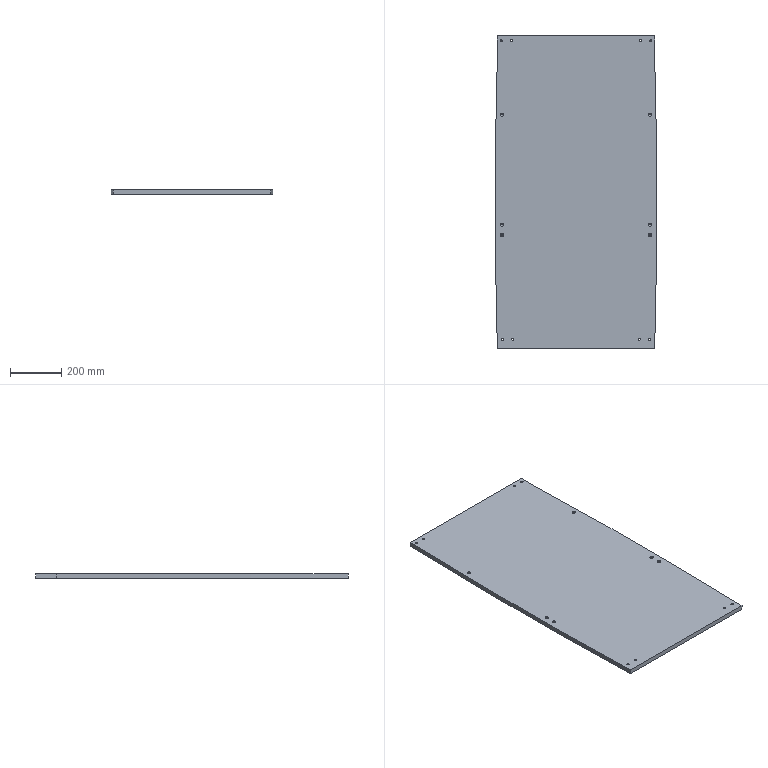Part | STEP file | DECAK 615 | 1 solid | 28 faces | box 633 x 1220 x 18 mm | volume 13739057 mm3 | cylinder 16 | plane 6 | cone 6 | commonest cylinder face diameters 8.5 x8 6.6 x6 36109 x2
STEP:
#1=CARTESIAN_POINT('',(307.5,530.,9.));
#2=VERTEX_POINT('',#1);
#3=CARTESIAN_POINT('',(307.5,610.,9.));
#4=VERTEX_POINT('',#3);
#5=CARTESIAN_POINT('',(307.5,610.,9.));
#6=DIRECTION('',(0.,1.,0.));
#7=VECTOR('',#6,1000.);
#8=LINE('',#5,#7);
#9=EDGE_CURVE('',#2,#4,#8,.T.);
#10=ORIENTED_EDGE('',*,*,#9,.F.);
#11=CARTESIAN_POINT('',(307.5,530.,-9.));
#12=VERTEX_POINT('',#11);
#13=CARTESIAN_POINT('',(307.5,530.,-1149.086));
#14=DIRECTION('',(0.,0.,1.));
#15=VECTOR('',#14,1000.);
#16=LINE('',#13,#15);
#17=EDGE_CURVE('',#12,#2,#16,.T.);
#18=ORIENTED_EDGE('',*,*,#17,.F.);
#19=CARTESIAN_POINT('',(307.5,610.,-9.));
#20=VERTEX_POINT('',#19);
#21=CARTESIAN_POINT('',(307.5,610.,-9.));
#22=DIRECTION('',(0.,1.,0.));
#23=VECTOR('',#22,1000.);
#24=LINE('',#21,#23);
#25=EDGE_CURVE('',#12,#20,#24,.T.);
#26=ORIENTED_EDGE('',*,*,#25,.T.);
#27=CARTESIAN_POINT('',(307.5,610.,9.));
#28=DIRECTION('',(0.,0.,-1.));
#29=VECTOR('',#28,1000.);
#30=LINE('',#27,#29);
#31=EDGE_CURVE('',#4,#20,#30,.T.);
#32=ORIENTED_EDGE('',*,*,#31,.F.);
#33=EDGE_LOOP('',(#10,#18,#26,#32));
#34=FACE_OUTER_BOUND('',#33,.T.);
#35=CARTESIAN_POINT('',(307.5,610.,9.));
#36=DIRECTION('',(-1.,0.,0.));
#37=DIRECTION('',(0.,0.,1.));
#38=AXIS2_PLACEMENT_3D('',#35,#36,#37);
#39=PLANE('',#38);
#40=ADVANCED_FACE('',(#34),#39,.F.);
#41=CARTESIAN_POINT('',(-307.5,610.,-9.));
#42=VERTEX_POINT('',#41);
#43=CARTESIAN_POINT('',(-307.5,610.,-9.));
#44=DIRECTION('',(-1.,0.,0.));
#45=VECTOR('',#44,1000.);
#46=LINE('',#43,#45);
#47=EDGE_CURVE('',#20,#42,#46,.T.);
#48=ORIENTED_EDGE('',*,*,#47,.T.);
#49=CARTESIAN_POINT('',(-307.5,610.,9.));
#50=VERTEX_POINT('',#49);
#51=CARTESIAN_POINT('',(-307.5,610.,9.));
#52=DIRECTION('',(0.,0.,-1.));
#53=VECTOR('',#52,1000.);
#54=LINE('',#51,#53);
#55=EDGE_CURVE('',#50,#42,#54,.T.);
#56=ORIENTED_EDGE('',*,*,#55,.F.);
#57=CARTESIAN_POINT('',(-307.5,610.,9.));
#58=DIRECTION('',(-1.,0.,0.));
#59=VECTOR('',#58,1000.);
#60=LINE('',#57,#59);
#61=EDGE_CURVE('',#4,#50,#60,.T.);
#62=ORIENTED_EDGE('',*,*,#61,.F.);
#63=ORIENTED_EDGE('',*,*,#31,.T.);
#64=EDGE_LOOP('',(#48,#56,#62,#63));
#65=FACE_OUTER_BOUND('',#64,.T.);
#66=CARTESIAN_POINT('',(-307.5,610.,9.));
#67=DIRECTION('',(0.,-1.,0.));
#68=DIRECTION('',(1.,0.,0.));
#69=AXIS2_PLACEMENT_3D('',#66,#67,#68);
#70=PLANE('',#69);
#71=ADVANCED_FACE('',(#65),#70,.F.);
#72=CARTESIAN_POINT('',(-307.5,530.,-9.));
#73=VERTEX_POINT('',#72);
#74=CARTESIAN_POINT('',(-307.5,610.,-9.));
#75=DIRECTION('',(0.,-1.,0.));
#76=VECTOR('',#75,1000.);
#77=LINE('',#74,#76);
#78=EDGE_CURVE('',#42,#73,#77,.T.);
#79=ORIENTED_EDGE('',*,*,#78,.T.);
#80=CARTESIAN_POINT('',(-307.5,530.,9.));
#81=VERTEX_POINT('',#80);
#82=CARTESIAN_POINT('',(-307.5,530.,-1149.086));
#83=DIRECTION('',(0.,0.,1.));
#84=VECTOR('',#83,1000.);
#85=LINE('',#82,#84);
#86=EDGE_CURVE('',#73,#81,#85,.T.);
#87=ORIENTED_EDGE('',*,*,#86,.T.);
#88=CARTESIAN_POINT('',(-307.5,610.,9.));
#89=DIRECTION('',(0.,-1.,0.));
#90=VECTOR('',#89,1000.);
#91=LINE('',#88,#90);
#92=EDGE_CURVE('',#50,#81,#91,.T.);
#93=ORIENTED_EDGE('',*,*,#92,.F.);
#94=ORIENTED_EDGE('',*,*,#55,.T.);
#95=EDGE_LOOP('',(#79,#87,#93,#94));
#96=FACE_OUTER_BOUND('',#95,.T.);
#97=CARTESIAN_POINT('',(-307.5,610.,9.));
#98=DIRECTION('',(1.,0.,0.));
#99=DIRECTION('',(0.,0.,-1.));
#100=AXIS2_PLACEMENT_3D('',#97,#98,#99);
#101=PLANE('',#100);
#102=ADVANCED_FACE('',(#96),#101,.F.);
#103=CARTESIAN_POINT('',(-307.5,-610.,-9.));
#104=VERTEX_POINT('',#103);
#105=CARTESIAN_POINT('',(307.5,-610.,-9.));
#106=VERTEX_POINT('',#105);
#107=CARTESIAN_POINT('',(-307.5,-610.,-9.));
#108=DIRECTION('',(1.,0.,0.));
#109=VECTOR('',#108,1000.);
#110=LINE('',#107,#109);
#111=EDGE_CURVE('',#104,#106,#110,.T.);
#112=ORIENTED_EDGE('',*,*,#111,.T.);
#113=CARTESIAN_POINT('',(307.5,-610.,9.));
#114=VERTEX_POINT('',#113);
#115=CARTESIAN_POINT('',(307.5,-610.,9.));
#116=DIRECTION('',(0.,0.,-1.));
#117=VECTOR('',#116,1000.);
#118=LINE('',#115,#117);
#119=EDGE_CURVE('',#114,#106,#118,.T.);
#120=ORIENTED_EDGE('',*,*,#119,.F.);
#121=CARTESIAN_POINT('',(-307.5,-610.,9.));
#122=VERTEX_POINT('',#121);
#123=CARTESIAN_POINT('',(-307.5,-610.,9.));
#124=DIRECTION('',(1.,0.,0.));
#125=VECTOR('',#124,1000.);
#126=LINE('',#123,#125);
#127=EDGE_CURVE('',#122,#114,#126,.T.);
#128=ORIENTED_EDGE('',*,*,#127,.F.);
#129=CARTESIAN_POINT('',(-307.5,-610.,9.));
#130=DIRECTION('',(0.,0.,-1.));
#131=VECTOR('',#130,1000.);
#132=LINE('',#129,#131);
#133=EDGE_CURVE('',#122,#104,#132,.T.);
#134=ORIENTED_EDGE('',*,*,#133,.T.);
#135=EDGE_LOOP('',(#112,#120,#128,#134));
#136=FACE_OUTER_BOUND('',#135,.T.);
#137=CARTESIAN_POINT('',(-307.5,-610.,9.));
#138=DIRECTION('',(0.,1.,0.));
#139=DIRECTION('',(-1.,0.,0.));
#140=AXIS2_PLACEMENT_3D('',#137,#138,#139);
#141=PLANE('',#140);
#142=ADVANCED_FACE('',(#136),#141,.F.);
#143=CARTESIAN_POINT('',(288.25,591.,9.));
#144=VERTEX_POINT('',#143);
#145=CARTESIAN_POINT('',(292.5,591.,9.));
#146=DIRECTION('',(0.,0.,1.));
#147=DIRECTION('',(-1.,0.,0.));
#148=AXIS2_PLACEMENT_3D('',#145,#146,#147);
#149=CIRCLE('',#148,4.25);
#150=EDGE_CURVE('',#144,#144,#149,.T.);
#151=ORIENTED_EDGE('',*,*,#150,.F.);
#152=EDGE_LOOP('',(#151));
#153=FACE_BOUND('',#152,.T.);
#154=CARTESIAN_POINT('',(248.25,591.,9.));
#155=VERTEX_POINT('',#154);
#156=CARTESIAN_POINT('',(252.5,591.,9.));
#157=DIRECTION('',(0.,0.,1.));
#158=DIRECTION('',(-1.,0.,0.));
#159=AXIS2_PLACEMENT_3D('',#156,#157,#158);
#160=CIRCLE('',#159,4.25);
#161=EDGE_CURVE('',#155,#155,#160,.T.);
#162=ORIENTED_EDGE('',*,*,#161,.F.);
#163=EDGE_LOOP('',(#162));
#164=FACE_BOUND('',#163,.T.);
#165=CARTESIAN_POINT('',(-248.25,591.,9.));
#166=VERTEX_POINT('',#165);
#167=CARTESIAN_POINT('',(-252.5,591.,9.));
#168=DIRECTION('',(0.,0.,1.));
#169=DIRECTION('',(1.,0.,0.));
#170=AXIS2_PLACEMENT_3D('',#167,#168,#169);
#171=CIRCLE('',#170,4.25);
#172=EDGE_CURVE('',#166,#166,#171,.T.);
#173=ORIENTED_EDGE('',*,*,#172,.F.);
#174=EDGE_LOOP('',(#173));
#175=FACE_BOUND('',#174,.T.);
#176=CARTESIAN_POINT('',(-288.25,591.,9.));
#177=VERTEX_POINT('',#176);
#178=CARTESIAN_POINT('',(-292.5,591.,9.));
#179=DIRECTION('',(0.,0.,1.));
#180=DIRECTION('',(1.,0.,0.));
#181=AXIS2_PLACEMENT_3D('',#178,#179,#180);
#182=CIRCLE('',#181,4.25);
#183=EDGE_CURVE('',#177,#177,#182,.T.);
#184=ORIENTED_EDGE('',*,*,#183,.F.);
#185=EDGE_LOOP('',(#184));
#186=FACE_BOUND('',#185,.T.);
#187=CARTESIAN_POINT('',(283.25,-575.,9.));
#188=VERTEX_POINT('',#187);
#189=CARTESIAN_POINT('',(287.5,-575.,9.));
#190=DIRECTION('',(0.,0.,1.));
#191=DIRECTION('',(-1.,0.,0.));
#192=AXIS2_PLACEMENT_3D('',#189,#190,#191);
#193=CIRCLE('',#192,4.25);
#194=EDGE_CURVE('',#188,#188,#193,.T.);
#195=ORIENTED_EDGE('',*,*,#194,.F.);
#196=EDGE_LOOP('',(#195));
#197=FACE_BOUND('',#196,.T.);
#198=CARTESIAN_POINT('',(243.25,-575.,9.));
#199=VERTEX_POINT('',#198);
#200=CARTESIAN_POINT('',(247.5,-575.,9.));
#201=DIRECTION('',(0.,0.,1.));
#202=DIRECTION('',(-1.,0.,0.));
#203=AXIS2_PLACEMENT_3D('',#200,#201,#202);
#204=CIRCLE('',#203,4.25);
#205=EDGE_CURVE('',#199,#199,#204,.T.);
#206=ORIENTED_EDGE('',*,*,#205,.F.);
#207=EDGE_LOOP('',(#206));
#208=FACE_BOUND('',#207,.T.);
#209=CARTESIAN_POINT('',(-243.25,-575.,9.));
#210=VERTEX_POINT('',#209);
#211=CARTESIAN_POINT('',(-247.5,-575.,9.));
#212=DIRECTION('',(0.,0.,1.));
#213=DIRECTION('',(1.,0.,0.));
#214=AXIS2_PLACEMENT_3D('',#211,#212,#213);
#215=CIRCLE('',#214,4.25);
#216=EDGE_CURVE('',#210,#210,#215,.T.);
#217=ORIENTED_EDGE('',*,*,#216,.F.);
#218=EDGE_LOOP('',(#217));
#219=FACE_BOUND('',#218,.T.);
#220=CARTESIAN_POINT('',(-283.25,-575.,9.));
#221=VERTEX_POINT('',#220);
#222=CARTESIAN_POINT('',(-287.5,-575.,9.));
#223=DIRECTION('',(0.,0.,1.));
#224=DIRECTION('',(1.,0.,0.));
#225=AXIS2_PLACEMENT_3D('',#222,#223,#224);
#226=CIRCLE('',#225,4.25);
#227=EDGE_CURVE('',#221,#221,#226,.T.);
#228=ORIENTED_EDGE('',*,*,#227,.F.);
#229=EDGE_LOOP('',(#228));
#230=FACE_BOUND('',#229,.T.);
#231=ORIENTED_EDGE('',*,*,#127,.T.);
#232=CARTESIAN_POINT('',(-17738.,-40.,9.));
#233=DIRECTION('',(0.,0.,1.));
#234=DIRECTION('',(-1.,0.,0.));
#235=AXIS2_PLACEMENT_3D('',#232,#233,#234);
#236=CIRCLE('',#235,18054.5);
#237=EDGE_CURVE('',#114,#2,#236,.T.);
#238=ORIENTED_EDGE('',*,*,#237,.T.);
#239=ORIENTED_EDGE('',*,*,#9,.T.);
#240=ORIENTED_EDGE('',*,*,#61,.T.);
#241=ORIENTED_EDGE('',*,*,#92,.T.);
#242=CARTESIAN_POINT('',(17738.,-40.,9.));
#243=DIRECTION('',(0.,0.,1.));
#244=DIRECTION('',(1.,0.,0.));
#245=AXIS2_PLACEMENT_3D('',#242,#243,#244);
#246=CIRCLE('',#245,18054.5);
#247=EDGE_CURVE('',#81,#122,#246,.T.);
#248=ORIENTED_EDGE('',*,*,#247,.T.);
#249=EDGE_LOOP('',(#231,#238,#239,#240,#241,#248));
#250=FACE_OUTER_BOUND('',#249,.T.);
#251=CARTESIAN_POINT('',(295.8,-168.,9.));
#252=VERTEX_POINT('',#251);
#253=CARTESIAN_POINT('',(289.5,-168.,9.));
#254=DIRECTION('',(0.,0.,-1.));
#255=DIRECTION('',(1.,0.,0.));
#256=AXIS2_PLACEMENT_3D('',#253,#254,#255);
#257=CIRCLE('',#256,6.3);
#258=EDGE_CURVE('',#252,#252,#257,.T.);
#259=ORIENTED_EDGE('',*,*,#258,.T.);
#260=EDGE_LOOP('',(#259));
#261=FACE_BOUND('',#260,.T.);
#262=CARTESIAN_POINT('',(-283.2,-168.,9.));
#263=VERTEX_POINT('',#262);
#264=CARTESIAN_POINT('',(-289.5,-168.,9.));
#265=DIRECTION('',(0.,0.,-1.));
#266=DIRECTION('',(1.,0.,0.));
#267=AXIS2_PLACEMENT_3D('',#264,#265,#266);
#268=CIRCLE('',#267,6.3);
#269=EDGE_CURVE('',#263,#263,#268,.T.);
#270=ORIENTED_EDGE('',*,*,#269,.T.);
#271=EDGE_LOOP('',(#270));
#272=FACE_BOUND('',#271,.T.);
#273=CARTESIAN_POINT('',(295.8,-128.,9.));
#274=VERTEX_POINT('',#273);
#275=CARTESIAN_POINT('',(289.5,-128.,9.));
#276=DIRECTION('',(0.,0.,-1.));
#277=DIRECTION('',(1.,0.,0.));
#278=AXIS2_PLACEMENT_3D('',#275,#276,#277);
#279=CIRCLE('',#278,6.3);
#280=EDGE_CURVE('',#274,#274,#279,.T.);
#281=ORIENTED_EDGE('',*,*,#280,.T.);
#282=EDGE_LOOP('',(#281));
#283=FACE_BOUND('',#282,.T.);
#284=CARTESIAN_POINT('',(295.8,302.,9.));
#285=VERTEX_POINT('',#284);
#286=CARTESIAN_POINT('',(289.5,302.,9.));
#287=DIRECTION('',(0.,0.,-1.));
#288=DIRECTION('',(1.,0.,0.));
#289=AXIS2_PLACEMENT_3D('',#286,#287,#288);
#290=CIRCLE('',#289,6.3);
#291=EDGE_CURVE('',#285,#285,#290,.T.);
#292=ORIENTED_EDGE('',*,*,#291,.T.);
#293=EDGE_LOOP('',(#292));
#294=FACE_BOUND('',#293,.T.);
#295=CARTESIAN_POINT('',(-283.2,-128.,9.));
#296=VERTEX_POINT('',#295);
#297=CARTESIAN_POINT('',(-289.5,-128.,9.));
#298=DIRECTION('',(0.,0.,-1.));
#299=DIRECTION('',(1.,0.,0.));
#300=AXIS2_PLACEMENT_3D('',#297,#298,#299);
#301=CIRCLE('',#300,6.3);
#302=EDGE_CURVE('',#296,#296,#301,.T.);
#303=ORIENTED_EDGE('',*,*,#302,.T.);
#304=EDGE_LOOP('',(#303));
#305=FACE_BOUND('',#304,.T.);
#306=CARTESIAN_POINT('',(-283.2,302.,9.));
#307=VERTEX_POINT('',#306);
#308=CARTESIAN_POINT('',(-289.5,302.,9.));
#309=DIRECTION('',(0.,0.,-1.));
#310=DIRECTION('',(1.,0.,0.));
#311=AXIS2_PLACEMENT_3D('',#308,#309,#310);
#312=CIRCLE('',#311,6.3);
#313=EDGE_CURVE('',#307,#307,#312,.T.);
#314=ORIENTED_EDGE('',*,*,#313,.T.);
#315=EDGE_LOOP('',(#314));
#316=FACE_BOUND('',#315,.T.);
#317=CARTESIAN_POINT('',(307.5,-610.,9.));
#318=DIRECTION('',(0.,0.,1.));
#319=DIRECTION('',(1.,0.,0.));
#320=AXIS2_PLACEMENT_3D('',#317,#318,#319);
#321=PLANE('',#320);
#322=ADVANCED_FACE('',(#153,#164,#175,#186,#197,#208,#219,#230,#250,#261,#272,#283,#294,#305,#316),#321,.T.);
#323=CARTESIAN_POINT('',(288.25,591.,-9.));
#324=VERTEX_POINT('',#323);
#325=CARTESIAN_POINT('',(292.5,591.,-9.));
#326=DIRECTION('',(0.,0.,1.));
#327=DIRECTION('',(-1.,0.,0.));
#328=AXIS2_PLACEMENT_3D('',#325,#326,#327);
#329=CIRCLE('',#328,4.25);
#330=EDGE_CURVE('',#324,#324,#329,.T.);
#331=ORIENTED_EDGE('',*,*,#330,.T.);
#332=EDGE_LOOP('',(#331));
#333=FACE_BOUND('',#332,.T.);
#334=CARTESIAN_POINT('',(248.25,591.,-9.));
#335=VERTEX_POINT('',#334);
#336=CARTESIAN_POINT('',(252.5,591.,-9.));
#337=DIRECTION('',(0.,0.,1.));
#338=DIRECTION('',(-1.,0.,0.));
#339=AXIS2_PLACEMENT_3D('',#336,#337,#338);
#340=CIRCLE('',#339,4.25);
#341=EDGE_CURVE('',#335,#335,#340,.T.);
#342=ORIENTED_EDGE('',*,*,#341,.T.);
#343=EDGE_LOOP('',(#342));
#344=FACE_BOUND('',#343,.T.);
#345=CARTESIAN_POINT('',(-248.25,591.,-9.));
#346=VERTEX_POINT('',#345);
#347=CARTESIAN_POINT('',(-252.5,591.,-9.));
#348=DIRECTION('',(0.,0.,1.));
#349=DIRECTION('',(1.,0.,0.));
#350=AXIS2_PLACEMENT_3D('',#347,#348,#349);
#351=CIRCLE('',#350,4.25);
#352=EDGE_CURVE('',#346,#346,#351,.T.);
#353=ORIENTED_EDGE('',*,*,#352,.T.);
#354=EDGE_LOOP('',(#353));
#355=FACE_BOUND('',#354,.T.);
#356=CARTESIAN_POINT('',(-288.25,591.,-9.));
#357=VERTEX_POINT('',#356);
#358=CARTESIAN_POINT('',(-292.5,591.,-9.));
#359=DIRECTION('',(0.,0.,1.));
#360=DIRECTION('',(1.,0.,0.));
#361=AXIS2_PLACEMENT_3D('',#358,#359,#360);
#362=CIRCLE('',#361,4.25);
#363=EDGE_CURVE('',#357,#357,#362,.T.);
#364=ORIENTED_EDGE('',*,*,#363,.T.);
#365=EDGE_LOOP('',(#364));
#366=FACE_BOUND('',#365,.T.);
#367=CARTESIAN_POINT('',(283.25,-575.,-9.));
#368=VERTEX_POINT('',#367);
#369=CARTESIAN_POINT('',(287.5,-575.,-9.));
#370=DIRECTION('',(0.,0.,1.));
#371=DIRECTION('',(-1.,0.,0.));
#372=AXIS2_PLACEMENT_3D('',#369,#370,#371);
#373=CIRCLE('',#372,4.25);
#374=EDGE_CURVE('',#368,#368,#373,.T.);
#375=ORIENTED_EDGE('',*,*,#374,.T.);
#376=EDGE_LOOP('',(#375));
#377=FACE_BOUND('',#376,.T.);
#378=CARTESIAN_POINT('',(243.25,-575.,-9.));
#379=VERTEX_POINT('',#378);
#380=CARTESIAN_POINT('',(247.5,-575.,-9.));
#381=DIRECTION('',(0.,0.,1.));
#382=DIRECTION('',(-1.,0.,0.));
#383=AXIS2_PLACEMENT_3D('',#380,#381,#382);
#384=CIRCLE('',#383,4.25);
#385=EDGE_CURVE('',#379,#379,#384,.T.);
#386=ORIENTED_EDGE('',*,*,#385,.T.);
#387=EDGE_LOOP('',(#386));
#388=FACE_BOUND('',#387,.T.);
#389=CARTESIAN_POINT('',(-243.25,-575.,-9.));
#390=VERTEX_POINT('',#389);
#391=CARTESIAN_POINT('',(-247.5,-575.,-9.));
#392=DIRECTION('',(0.,0.,1.));
#393=DIRECTION('',(1.,0.,0.));
#394=AXIS2_PLACEMENT_3D('',#391,#392,#393);
#395=CIRCLE('',#394,4.25);
#396=EDGE_CURVE('',#390,#390,#395,.T.);
#397=ORIENTED_EDGE('',*,*,#396,.T.);
#398=EDGE_LOOP('',(#397));
#399=FACE_BOUND('',#398,.T.);
#400=CARTESIAN_POINT('',(-283.25,-575.,-9.));
#401=VERTEX_POINT('',#400);
#402=CARTESIAN_POINT('',(-287.5,-575.,-9.));
#403=DIRECTION('',(0.,0.,1.));
#404=DIRECTION('',(1.,0.,0.));
#405=AXIS2_PLACEMENT_3D('',#402,#403,#404);
#406=CIRCLE('',#405,4.25);
#407=EDGE_CURVE('',#401,#401,#406,.T.);
#408=ORIENTED_EDGE('',*,*,#407,.T.);
#409=EDGE_LOOP('',(#408));
#410=FACE_BOUND('',#409,.T.);
#411=CARTESIAN_POINT('',(-17738.,-40.,-9.));
#412=DIRECTION('',(0.,0.,-1.));
#413=DIRECTION('',(1.,0.,0.));
#414=AXIS2_PLACEMENT_3D('',#411,#412,#413);
#415=CIRCLE('',#414,18054.5);
#416=EDGE_CURVE('',#12,#106,#415,.T.);
#417=ORIENTED_EDGE('',*,*,#416,.T.);
#418=ORIENTED_EDGE('',*,*,#111,.F.);
#419=CARTESIAN_POINT('',(17738.,-40.,-9.));
#420=DIRECTION('',(0.,0.,-1.));
#421=DIRECTION('',(1.,0.,0.));
#422=AXIS2_PLACEMENT_3D('',#419,#420,#421);
#423=CIRCLE('',#422,18054.5);
#424=EDGE_CURVE('',#104,#73,#423,.T.);
#425=ORIENTED_EDGE('',*,*,#424,.T.);
#426=ORIENTED_EDGE('',*,*,#78,.F.);
#427=ORIENTED_EDGE('',*,*,#47,.F.);
#428=ORIENTED_EDGE('',*,*,#25,.F.);
#429=EDGE_LOOP('',(#417,#418,#425,#426,#427,#428));
#430=FACE_OUTER_BOUND('',#429,.T.);
#431=CARTESIAN_POINT('',(286.2,-168.,-9.));
#432=VERTEX_POINT('',#431);
#433=CARTESIAN_POINT('',(289.5,-168.,-9.));
#434=DIRECTION('',(0.,0.,1.));
#435=DIRECTION('',(-1.,0.,0.));
#436=AXIS2_PLACEMENT_3D('',#433,#434,#435);
#437=CIRCLE('',#436,3.3);
#438=EDGE_CURVE('',#432,#432,#437,.T.);
#439=ORIENTED_EDGE('',*,*,#438,.T.);
#440=EDGE_LOOP('',(#439));
#441=FACE_BOUND('',#440,.T.);
#442=CARTESIAN_POINT('',(286.2,302.,-9.));
#443=VERTEX_POINT('',#442);
#444=CARTESIAN_POINT('',(289.5,302.,-9.));
#445=DIRECTION('',(0.,0.,1.));
#446=DIRECTION('',(-1.,0.,0.));
#447=AXIS2_PLACEMENT_3D('',#444,#445,#446);
#448=CIRCLE('',#447,3.3);
#449=EDGE_CURVE('',#443,#443,#448,.T.);
#450=ORIENTED_EDGE('',*,*,#449,.T.);
#451=EDGE_LOOP('',(#450));
#452=FACE_BOUND('',#451,.T.);
#453=CARTESIAN_POINT('',(286.2,-128.,-9.));
#454=VERTEX_POINT('',#453);
#455=CARTESIAN_POINT('',(289.5,-128.,-9.));
#456=DIRECTION('',(0.,0.,1.));
#457=DIRECTION('',(-1.,0.,0.));
#458=AXIS2_PLACEMENT_3D('',#455,#456,#457);
#459=CIRCLE('',#458,3.3);
#460=EDGE_CURVE('',#454,#454,#459,.T.);
#461=ORIENTED_EDGE('',*,*,#460,.T.);
#462=EDGE_LOOP('',(#461));
#463=FACE_BOUND('',#462,.T.);
#464=CARTESIAN_POINT('',(-286.2,-168.,-9.));
#465=VERTEX_POINT('',#464);
#466=CARTESIAN_POINT('',(-289.5,-168.,-9.));
#467=DIRECTION('',(0.,0.,1.));
#468=DIRECTION('',(1.,0.,0.));
#469=AXIS2_PLACEMENT_3D('',#466,#467,#468);
#470=CIRCLE('',#469,3.3);
#471=EDGE_CURVE('',#465,#465,#470,.T.);
#472=ORIENTED_EDGE('',*,*,#471,.T.);
#473=EDGE_LOOP('',(#472));
#474=FACE_BOUND('',#473,.T.);
#475=CARTESIAN_POINT('',(-286.2,-128.,-9.));
#476=VERTEX_POINT('',#475);
#477=CARTESIAN_POINT('',(-289.5,-128.,-9.));
#478=DIRECTION('',(0.,0.,1.));
#479=DIRECTION('',(1.,0.,0.));
#480=AXIS2_PLACEMENT_3D('',#477,#478,#479);
#481=CIRCLE('',#480,3.3);
#482=EDGE_CURVE('',#476,#476,#481,.T.);
#483=ORIENTED_EDGE('',*,*,#482,.T.);
#484=EDGE_LOOP('',(#483));
#485=FACE_BOUND('',#484,.T.);
#486=CARTESIAN_POINT('',(-286.2,302.,-9.));
#487=VERTEX_POINT('',#486);
#488=CARTESIAN_POINT('',(-289.5,302.,-9.));
#489=DIRECTION('',(0.,0.,1.));
#490=DIRECTION('',(1.,0.,0.));
#491=AXIS2_PLACEMENT_3D('',#488,#489,#490);
#492=CIRCLE('',#491,3.3);
#493=EDGE_CURVE('',#487,#487,#492,.T.);
#494=ORIENTED_EDGE('',*,*,#493,.T.);
#495=EDGE_LOOP('',(#494));
#496=FACE_BOUND('',#495,.T.);
#497=CARTESIAN_POINT('',(307.5,-610.,-9.));
#498=DIRECTION('',(0.,0.,1.));
#499=DIRECTION('',(1.,0.,0.));
#500=AXIS2_PLACEMENT_3D('',#497,#498,#499);
#501=PLANE('',#500);
#502=ADVANCED_FACE('',(#333,#344,#355,#366,#377,#388,#399,#410,#430,#441,#452,#463,#474,#485,#496),#501,.F.);
#503=CARTESIAN_POINT('',(-286.2,302.,6.));
#504=VERTEX_POINT('',#503);
#505=CARTESIAN_POINT('',(-289.5,302.,6.));
#506=DIRECTION('',(0.,0.,1.));
#507=DIRECTION('',(1.,0.,0.));
#508=AXIS2_PLACEMENT_3D('',#505,#506,#507);
#509=CIRCLE('',#508,3.3);
#510=EDGE_CURVE('',#504,#504,#509,.T.);
#511=ORIENTED_EDGE('',*,*,#510,.T.);
#512=EDGE_LOOP('',(#511));
#513=FACE_OUTER_BOUND('',#512,.T.);
#514=ORIENTED_EDGE('',*,*,#493,.F.);
#515=EDGE_LOOP('',(#514));
#516=FACE_OUTER_BOUND('',#515,.T.);
#517=CARTESIAN_POINT('',(-289.5,302.,-9.));
#518=DIRECTION('',(0.,0.,1.));
#519=DIRECTION('',(1.,0.,0.));
#520=AXIS2_PLACEMENT_3D('',#517,#518,#519);
#521=CYLINDRICAL_SURFACE('',#520,3.3);
#522=ADVANCED_FACE('',(#513,#516),#521,.F.);
#523=CARTESIAN_POINT('',(-286.2,-128.,6.));
#524=VERTEX_POINT('',#523);
#525=CARTESIAN_POINT('',(-289.5,-128.,6.));
#526=DIRECTION('',(0.,0.,1.));
#527=DIRECTION('',(1.,0.,0.));
#528=AXIS2_PLACEMENT_3D('',#525,#526,#527);
#529=CIRCLE('',#528,3.3);
#530=EDGE_CURVE('',#524,#524,#529,.T.);
#531=ORIENTED_EDGE('',*,*,#530,.T.);
#532=EDGE_LOOP('',(#531));
#533=FACE_OUTER_BOUND('',#532,.T.);
#534=ORIENTED_EDGE('',*,*,#482,.F.);
#535=EDGE_LOOP('',(#534));
#536=FACE_OUTER_BOUND('',#535,.T.);
#537=CARTESIAN_POINT('',(-289.5,-128.,-9.));
#538=DIRECTION('',(0.,0.,1.));
#539=DIRECTION('',(1.,0.,0.));
#540=AXIS2_PLACEMENT_3D('',#537,#538,#539);
#541=CYLINDRICAL_SURFACE('',#540,3.3);
#542=ADVANCED_FACE('',(#533,#536),#541,.F.);
#543=CARTESIAN_POINT('',(-286.2,-168.,6.));
#544=VERTEX_POINT('',#543);
#545=CARTESIAN_POINT('',(-289.5,-168.,6.));
#546=DIRECTION('',(0.,0.,1.));
#547=DIRECTION('',(1.,0.,0.));
#548=AXIS2_PLACEMENT_3D('',#545,#546,#547);
#549=CIRCLE('',#548,3.3);
#550=EDGE_CURVE('',#544,#544,#549,.T.);
#551=ORIENTED_EDGE('',*,*,#550,.T.);
#552=EDGE_LOOP('',(#551));
#553=FACE_OUTER_BOUND('',#552,.T.);
#554=ORIENTED_EDGE('',*,*,#471,.F.);
#555=EDGE_LOOP('',(#554));
#556=FACE_OUTER_BOUND('',#555,.T.);
#557=CARTESIAN_POINT('',(-289.5,-168.,-9.));
#558=DIRECTION('',(0.,0.,1.));
#559=DIRECTION('',(1.,0.,0.));
#560=AXIS2_PLACEMENT_3D('',#557,#558,#559);
#561=CYLINDRICAL_SURFACE('',#560,3.3);
#562=ADVANCED_FACE('',(#553,#556),#561,.F.);
#563=CARTESIAN_POINT('',(292.8,-128.,6.));
#564=VERTEX_POINT('',#563);
#565=CARTESIAN_POINT('',(289.5,-128.,6.));
#566=DIRECTION('',(0.,0.,1.));
#567=DIRECTION('',(1.,0.,0.));
#568=AXIS2_PLACEMENT_3D('',#565,#566,#567);
#569=CIRCLE('',#568,3.3);
#570=EDGE_CURVE('',#564,#564,#569,.T.);
#571=ORIENTED_EDGE('',*,*,#570,.T.);
#572=EDGE_LOOP('',(#571));
#573=FACE_OUTER_BOUND('',#572,.T.);
#574=ORIENTED_EDGE('',*,*,#460,.F.);
#575=EDGE_LOOP('',(#574));
#576=FACE_OUTER_BOUND('',#575,.T.);
#577=CARTESIAN_POINT('',(289.5,-128.,-9.));
#578=DIRECTION('',(0.,0.,1.));
#579=DIRECTION('',(1.,0.,0.));
#580=AXIS2_PLACEMENT_3D('',#577,#578,#579);
#581=CYLINDRICAL_SURFACE('',#580,3.3);
#582=ADVANCED_FACE('',(#573,#576),#581,.F.);
#583=CARTESIAN_POINT('',(292.8,302.,6.));
#584=VERTEX_POINT('',#583);
#585=CARTESIAN_POINT('',(289.5,302.,6.));
#586=DIRECTION('',(0.,0.,1.));
#587=DIRECTION('',(1.,0.,0.));
#588=AXIS2_PLACEMENT_3D('',#585,#586,#587);
#589=CIRCLE('',#588,3.3);
#590=EDGE_CURVE('',#584,#584,#589,.T.);
#591=ORIENTED_EDGE('',*,*,#590,.T.);
#592=EDGE_LOOP('',(#591));
#593=FACE_OUTER_BOUND('',#592,.T.);
#594=ORIENTED_EDGE('',*,*,#449,.F.);
#595=EDGE_LOOP('',(#594));
#596=FACE_OUTER_BOUND('',#595,.T.);
#597=CARTESIAN_POINT('',(289.5,302.,-9.));
#598=DIRECTION('',(0.,0.,1.));
#599=DIRECTION('',(1.,0.,0.));
#600=AXIS2_PLACEMENT_3D('',#597,#598,#599);
#601=CYLINDRICAL_SURFACE('',#600,3.3);
#602=ADVANCED_FACE('',(#593,#596),#601,.F.);
#603=CARTESIAN_POINT('',(292.8,-168.,6.));
#604=VERTEX_POINT('',#603);
#605=CARTESIAN_POINT('',(289.5,-168.,6.));
#606=DIRECTION('',(0.,0.,1.));
#607=DIRECTION('',(1.,0.,0.));
#608=AXIS2_PLACEMENT_3D('',#605,#606,#607);
#609=CIRCLE('',#608,3.3);
#610=EDGE_CURVE('',#604,#604,#609,.T.);
#611=ORIENTED_EDGE('',*,*,#610,.T.);
#612=EDGE_LOOP('',(#611));
#613=FACE_OUTER_BOUND('',#612,.T.);
#614=ORIENTED_EDGE('',*,*,#438,.F.);
#615=EDGE_LOOP('',(#614));
#616=FACE_OUTER_BOUND('',#615,.T.);
#617=CARTESIAN_POINT('',(289.5,-168.,-9.));
#618=DIRECTION('',(0.,0.,1.));
#619=DIRECTION('',(1.,0.,0.));
#620=AXIS2_PLACEMENT_3D('',#617,#618,#619);
#621=CYLINDRICAL_SURFACE('',#620,3.3);
#622=ADVANCED_FACE('',(#613,#616),#621,.F.);
#623=ORIENTED_EDGE('',*,*,#258,.F.);
#624=EDGE_LOOP('',(#623));
#625=FACE_OUTER_BOUND('',#624,.T.);
#626=ORIENTED_EDGE('',*,*,#610,.F.);
#627=EDGE_LOOP('',(#626));
#628=FACE_BOUND('',#627,.T.);
#629=CARTESIAN_POINT('',(289.5,-168.,6.));
#630=DIRECTION('',(0.,0.,1.));
#631=DIRECTION('',(1.,0.,0.));
#632=AXIS2_PLACEMENT_3D('',#629,#630,#631);
#633=CONICAL_SURFACE('',#632,3.3,0.7854);
#634=ADVANCED_FACE('',(#625,#628),#633,.F.);
#635=ORIENTED_EDGE('',*,*,#269,.F.);
#636=EDGE_LOOP('',(#635));
#637=FACE_OUTER_BOUND('',#636,.T.);
#638=ORIENTED_EDGE('',*,*,#550,.F.);
#639=EDGE_LOOP('',(#638));
#640=FACE_BOUND('',#639,.T.);
#641=CARTESIAN_POINT('',(-289.5,-168.,6.));
#642=DIRECTION('',(0.,0.,1.));
#643=DIRECTION('',(1.,0.,0.));
#644=AXIS2_PLACEMENT_3D('',#641,#642,#643);
#645=CONICAL_SURFACE('',#644,3.3,0.7854);
#646=ADVANCED_FACE('',(#637,#640),#645,.F.);
#647=ORIENTED_EDGE('',*,*,#280,.F.);
#648=EDGE_LOOP('',(#647));
#649=FACE_OUTER_BOUND('',#648,.T.);
#650=ORIENTED_EDGE('',*,*,#570,.F.);
#651=EDGE_LOOP('',(#650));
#652=FACE_BOUND('',#651,.T.);
#653=CARTESIAN_POINT('',(289.5,-128.,6.));
#654=DIRECTION('',(0.,0.,1.));
#655=DIRECTION('',(1.,0.,0.));
#656=AXIS2_PLACEMENT_3D('',#653,#654,#655);
#657=CONICAL_SURFACE('',#656,3.3,0.7854);
#658=ADVANCED_FACE('',(#649,#652),#657,.F.);
#659=ORIENTED_EDGE('',*,*,#291,.F.);
#660=EDGE_LOOP('',(#659));
#661=FACE_OUTER_BOUND('',#660,.T.);
#662=ORIENTED_EDGE('',*,*,#590,.F.);
#663=EDGE_LOOP('',(#662));
#664=FACE_BOUND('',#663,.T.);
#665=CARTESIAN_POINT('',(289.5,302.,6.));
#666=DIRECTION('',(0.,0.,1.));
#667=DIRECTION('',(1.,0.,0.));
#668=AXIS2_PLACEMENT_3D('',#665,#666,#667);
#669=CONICAL_SURFACE('',#668,3.3,0.7854);
#670=ADVANCED_FACE('',(#661,#664),#669,.F.);
#671=ORIENTED_EDGE('',*,*,#302,.F.);
#672=EDGE_LOOP('',(#671));
#673=FACE_OUTER_BOUND('',#672,.T.);
#674=ORIENTED_EDGE('',*,*,#530,.F.);
#675=EDGE_LOOP('',(#674));
#676=FACE_BOUND('',#675,.T.);
#677=CARTESIAN_POINT('',(-289.5,-128.,6.));
#678=DIRECTION('',(0.,0.,1.));
#679=DIRECTION('',(1.,0.,0.));
#680=AXIS2_PLACEMENT_3D('',#677,#678,#679);
#681=CONICAL_SURFACE('',#680,3.3,0.7854);
#682=ADVANCED_FACE('',(#673,#676),#681,.F.);
#683=ORIENTED_EDGE('',*,*,#313,.F.);
#684=EDGE_LOOP('',(#683));
#685=FACE_OUTER_BOUND('',#684,.T.);
#686=ORIENTED_EDGE('',*,*,#510,.F.);
#687=EDGE_LOOP('',(#686));
#688=FACE_BOUND('',#687,.T.);
#689=CARTESIAN_POINT('',(-289.5,302.,6.));
#690=DIRECTION('',(0.,0.,1.));
#691=DIRECTION('',(1.,0.,0.));
#692=AXIS2_PLACEMENT_3D('',#689,#690,#691);
#693=CONICAL_SURFACE('',#692,3.3,0.7854);
#694=ADVANCED_FACE('',(#685,#688),#693,.F.);
#695=ORIENTED_EDGE('',*,*,#424,.F.);
#696=ORIENTED_EDGE('',*,*,#133,.F.);
#697=ORIENTED_EDGE('',*,*,#247,.F.);
#698=ORIENTED_EDGE('',*,*,#86,.F.);
#699=EDGE_LOOP('',(#695,#696,#697,#698));
#700=FACE_OUTER_BOUND('',#699,.T.);
#701=CARTESIAN_POINT('',(17738.,-40.,-1149.086));
#702=DIRECTION('',(0.,0.,1.));
#703=DIRECTION('',(1.,0.,0.));
#704=AXIS2_PLACEMENT_3D('',#701,#702,#703);
#705=CYLINDRICAL_SURFACE('',#704,18054.5);
#706=ADVANCED_FACE('',(#700),#705,.T.);
#707=ORIENTED_EDGE('',*,*,#416,.F.);
#708=ORIENTED_EDGE('',*,*,#17,.T.);
#709=ORIENTED_EDGE('',*,*,#237,.F.);
#710=ORIENTED_EDGE('',*,*,#119,.T.);
#711=EDGE_LOOP('',(#707,#708,#709,#710));
#712=FACE_OUTER_BOUND('',#711,.T.);
#713=CARTESIAN_POINT('',(-17738.,-40.,-1149.086));
#714=DIRECTION('',(0.,0.,1.));
#715=DIRECTION('',(1.,0.,0.));
#716=AXIS2_PLACEMENT_3D('',#713,#714,#715);
#717=CYLINDRICAL_SURFACE('',#716,18054.5);
#718=ADVANCED_FACE('',(#712),#717,.T.);
#719=ORIENTED_EDGE('',*,*,#407,.F.);
#720=EDGE_LOOP('',(#719));
#721=FACE_OUTER_BOUND('',#720,.T.);
#722=ORIENTED_EDGE('',*,*,#227,.T.);
#723=EDGE_LOOP('',(#722));
#724=FACE_OUTER_BOUND('',#723,.T.);
#725=CARTESIAN_POINT('',(-287.5,-575.,-9.));
#726=DIRECTION('',(0.,0.,1.));
#727=DIRECTION('',(1.,0.,0.));
#728=AXIS2_PLACEMENT_3D('',#725,#726,#727);
#729=CYLINDRICAL_SURFACE('',#728,4.25);
#730=ADVANCED_FACE('',(#721,#724),#729,.F.);
#731=ORIENTED_EDGE('',*,*,#396,.F.);
#732=EDGE_LOOP('',(#731));
#733=FACE_OUTER_BOUND('',#732,.T.);
#734=ORIENTED_EDGE('',*,*,#216,.T.);
#735=EDGE_LOOP('',(#734));
#736=FACE_OUTER_BOUND('',#735,.T.);
#737=CARTESIAN_POINT('',(-247.5,-575.,-9.));
#738=DIRECTION('',(0.,0.,1.));
#739=DIRECTION('',(1.,0.,0.));
#740=AXIS2_PLACEMENT_3D('',#737,#738,#739);
#741=CYLINDRICAL_SURFACE('',#740,4.25);
#742=ADVANCED_FACE('',(#733,#736),#741,.F.);
#743=ORIENTED_EDGE('',*,*,#385,.F.);
#744=EDGE_LOOP('',(#743));
#745=FACE_OUTER_BOUND('',#744,.T.);
#746=ORIENTED_EDGE('',*,*,#205,.T.);
#747=EDGE_LOOP('',(#746));
#748=FACE_OUTER_BOUND('',#747,.T.);
#749=CARTESIAN_POINT('',(247.5,-575.,-9.));
#750=DIRECTION('',(0.,0.,1.));
#751=DIRECTION('',(1.,0.,0.));
#752=AXIS2_PLACEMENT_3D('',#749,#750,#751);
#753=CYLINDRICAL_SURFACE('',#752,4.25);
#754=ADVANCED_FACE('',(#745,#748),#753,.F.);
#755=ORIENTED_EDGE('',*,*,#374,.F.);
#756=EDGE_LOOP('',(#755));
#757=FACE_OUTER_BOUND('',#756,.T.);
#758=ORIENTED_EDGE('',*,*,#194,.T.);
#759=EDGE_LOOP('',(#758));
#760=FACE_OUTER_BOUND('',#759,.T.);
#761=CARTESIAN_POINT('',(287.5,-575.,-9.));
#762=DIRECTION('',(0.,0.,1.));
#763=DIRECTION('',(1.,0.,0.));
#764=AXIS2_PLACEMENT_3D('',#761,#762,#763);
#765=CYLINDRICAL_SURFACE('',#764,4.25);
#766=ADVANCED_FACE('',(#757,#760),#765,.F.);
#767=ORIENTED_EDGE('',*,*,#363,.F.);
#768=EDGE_LOOP('',(#767));
#769=FACE_OUTER_BOUND('',#768,.T.);
#770=ORIENTED_EDGE('',*,*,#183,.T.);
#771=EDGE_LOOP('',(#770));
#772=FACE_OUTER_BOUND('',#771,.T.);
#773=CARTESIAN_POINT('',(-292.5,591.,-9.));
#774=DIRECTION('',(0.,0.,1.));
#775=DIRECTION('',(1.,0.,0.));
#776=AXIS2_PLACEMENT_3D('',#773,#774,#775);
#777=CYLINDRICAL_SURFACE('',#776,4.25);
#778=ADVANCED_FACE('',(#769,#772),#777,.F.);
#779=ORIENTED_EDGE('',*,*,#352,.F.);
#780=EDGE_LOOP('',(#779));
#781=FACE_OUTER_BOUND('',#780,.T.);
#782=ORIENTED_EDGE('',*,*,#172,.T.);
#783=EDGE_LOOP('',(#782));
#784=FACE_OUTER_BOUND('',#783,.T.);
#785=CARTESIAN_POINT('',(-252.5,591.,-9.));
#786=DIRECTION('',(0.,0.,1.));
#787=DIRECTION('',(1.,0.,0.));
#788=AXIS2_PLACEMENT_3D('',#785,#786,#787);
#789=CYLINDRICAL_SURFACE('',#788,4.25);
#790=ADVANCED_FACE('',(#781,#784),#789,.F.);
#791=ORIENTED_EDGE('',*,*,#341,.F.);
#792=EDGE_LOOP('',(#791));
#793=FACE_OUTER_BOUND('',#792,.T.);
#794=ORIENTED_EDGE('',*,*,#161,.T.);
#795=EDGE_LOOP('',(#794));
#796=FACE_OUTER_BOUND('',#795,.T.);
#797=CARTESIAN_POINT('',(252.5,591.,-9.));
#798=DIRECTION('',(0.,0.,1.));
#799=DIRECTION('',(1.,0.,0.));
#800=AXIS2_PLACEMENT_3D('',#797,#798,#799);
#801=CYLINDRICAL_SURFACE('',#800,4.25);
#802=ADVANCED_FACE('',(#793,#796),#801,.F.);
#803=ORIENTED_EDGE('',*,*,#330,.F.);
#804=EDGE_LOOP('',(#803));
#805=FACE_OUTER_BOUND('',#804,.T.);
#806=ORIENTED_EDGE('',*,*,#150,.T.);
#807=EDGE_LOOP('',(#806));
#808=FACE_OUTER_BOUND('',#807,.T.);
#809=CARTESIAN_POINT('',(292.5,591.,-9.));
#810=DIRECTION('',(0.,0.,1.));
#811=DIRECTION('',(1.,0.,0.));
#812=AXIS2_PLACEMENT_3D('',#809,#810,#811);
#813=CYLINDRICAL_SURFACE('',#812,4.25);
#814=ADVANCED_FACE('',(#805,#808),#813,.F.);
#815=CLOSED_SHELL('',(#40,#71,#102,#142,#322,#502,#522,#542,#562,#582,#602,#622,#634,#646,#658,#670,#682,#694,#706,#718,#730,#742,#754,#766,#778,#790,#802,#814));
#816=MANIFOLD_SOLID_BREP('',#815);
#817=CARTESIAN_POINT('',(0.,0.,0.));
#818=DIRECTION('',(0.,0.,1.));
#819=DIRECTION('',(1.,0.,0.));
#820=AXIS2_PLACEMENT_3D('',#817,#818,#819);
#821=(LENGTH_UNIT()NAMED_UNIT(*)SI_UNIT(.MILLI.,.METRE.));
#822=UNCERTAINTY_MEASURE_WITH_UNIT(LENGTH_MEASURE(0.00001),#821,'','');
#823=(NAMED_UNIT(*)PLANE_ANGLE_UNIT()SI_UNIT($,.RADIAN.));
#824=(NAMED_UNIT(*)SI_UNIT($,.STERADIAN.)SOLID_ANGLE_UNIT());
#825=(GEOMETRIC_REPRESENTATION_CONTEXT(3)GLOBAL_UNCERTAINTY_ASSIGNED_CONTEXT((#822))GLOBAL_UNIT_ASSIGNED_CONTEXT((#821,#823,#824))REPRESENTATION_CONTEXT('',''));
#826=ADVANCED_BREP_SHAPE_REPRESENTATION('',(#816,#820),#825);